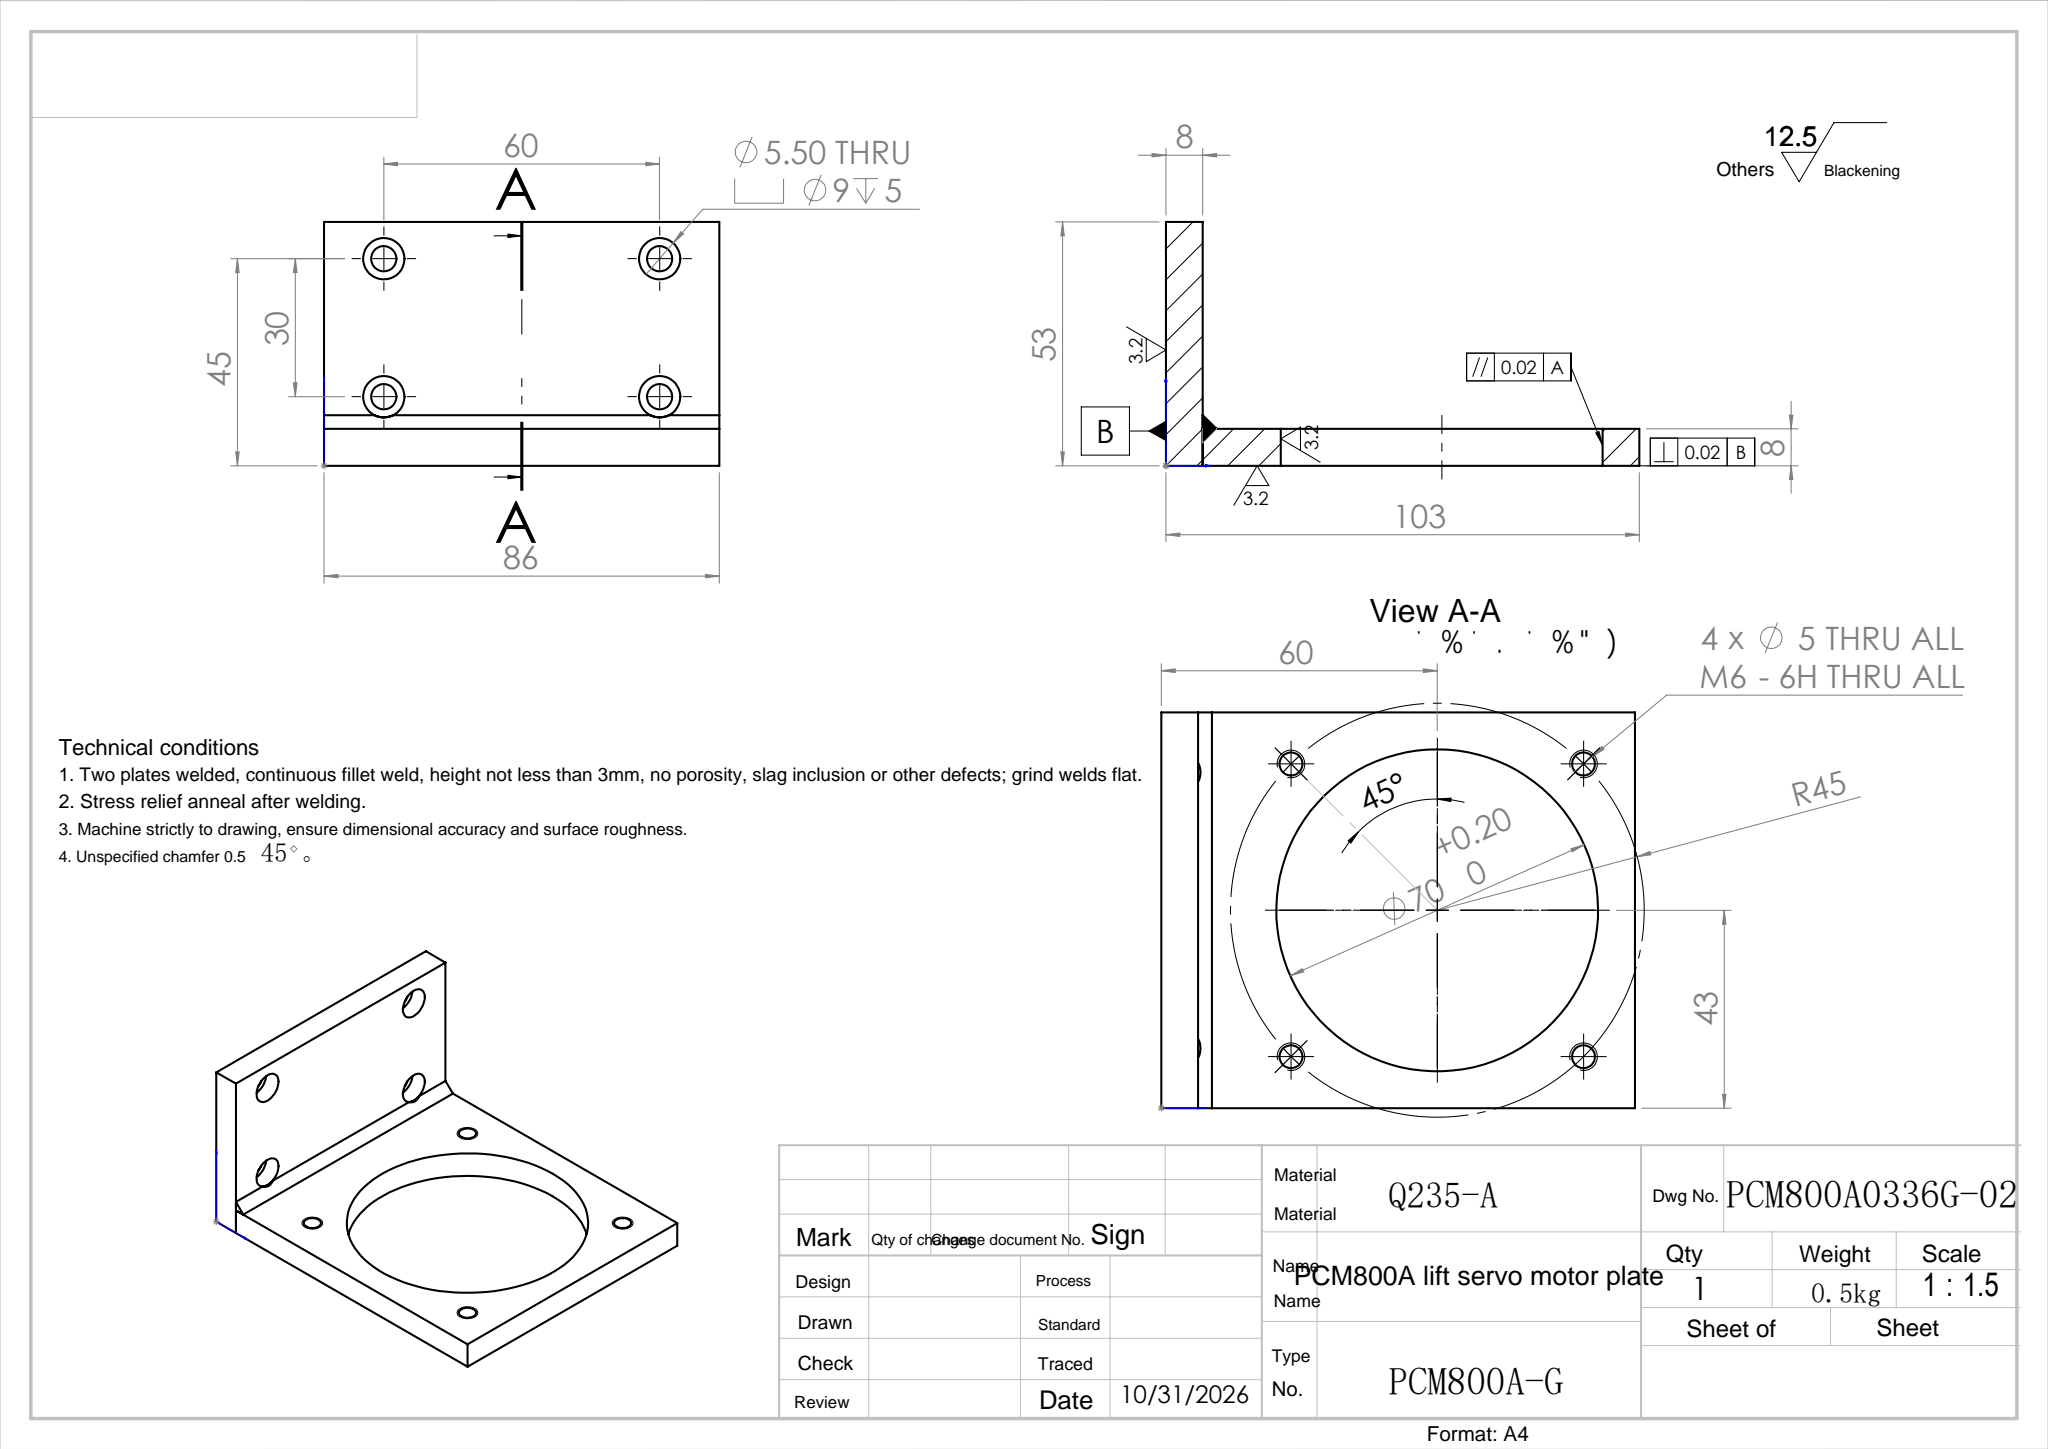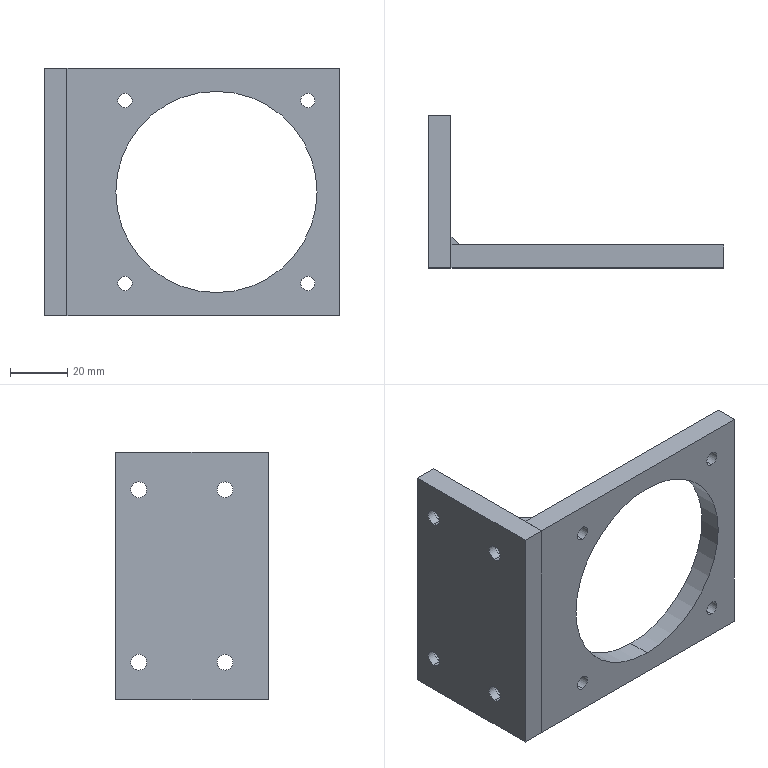Part | SolidWorks | features HoleWzd 2, 3DProfileFeature 1, Boss 1, Extrusion 1, ICE 1, Split 1, WeldBeadFeat 1, WeldmentFeature 1 | 3 solids | 49 faces | box 103 x 53 x 86 mm | volume 69237 mm3 | cylinder 28 | plane 21 | commonest cylinder face diameters 9 x10 5 x8 5.5 x8 70 x2